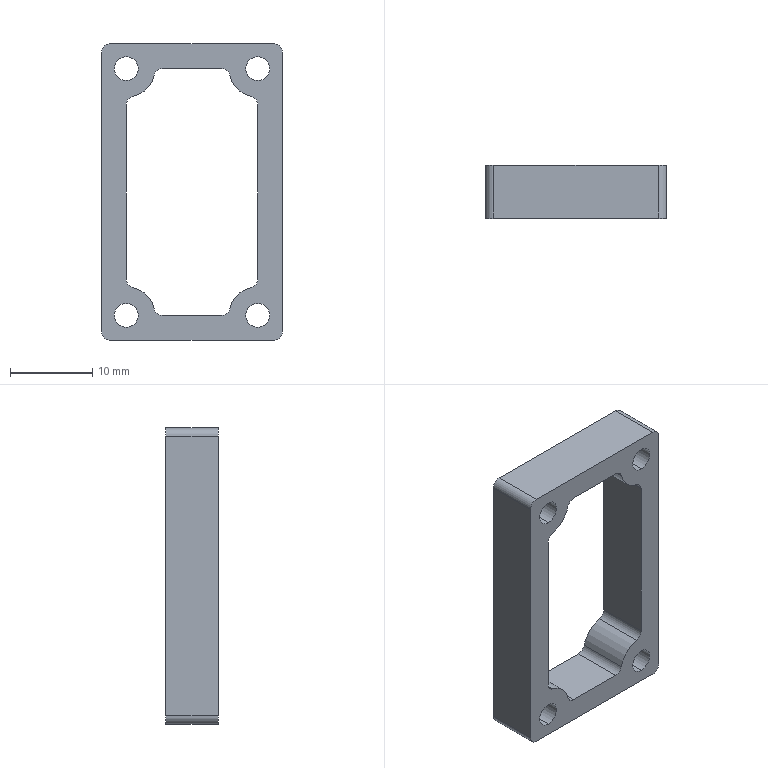Part | SolidWorks | features Fillet 2, Extrusion 1 | 1 solid | 34 faces | box 22 x 6.4 x 36 mm | volume 2076 mm3 | cylinder 24 | plane 10 | commonest cylinder face diameters 2 x12 2.9 x8 7 x4
STEP:
#1=CARTESIAN_POINT('',(8.,6.4,13.55));
#2=VERTEX_POINT('',#1);
#3=CARTESIAN_POINT('',(8.,6.4,16.45));
#4=VERTEX_POINT('',#3);
#5=CARTESIAN_POINT('',(8.,6.4,15.));
#6=DIRECTION('',(0.,1.,0.));
#7=DIRECTION('',(0.,0.,1.));
#8=AXIS2_PLACEMENT_3D('',#5,#6,#7);
#9=CIRCLE('',#8,1.45);
#10=EDGE_CURVE('',#2,#4,#9,.T.);
#11=ORIENTED_EDGE('',*,*,#10,.T.);
#12=CARTESIAN_POINT('',(8.,0.,16.45));
#13=VERTEX_POINT('',#12);
#14=CARTESIAN_POINT('',(8.,6.4,16.45));
#15=DIRECTION('',(0.,-1.,0.));
#16=VECTOR('',#15,1000.);
#17=LINE('',#14,#16);
#18=EDGE_CURVE('',#4,#13,#17,.T.);
#19=ORIENTED_EDGE('',*,*,#18,.T.);
#20=CARTESIAN_POINT('',(8.,0.,13.55));
#21=VERTEX_POINT('',#20);
#22=CARTESIAN_POINT('',(8.,0.,15.));
#23=DIRECTION('',(0.,1.,0.));
#24=DIRECTION('',(0.,0.,1.));
#25=AXIS2_PLACEMENT_3D('',#22,#23,#24);
#26=CIRCLE('',#25,1.45);
#27=EDGE_CURVE('',#21,#13,#26,.T.);
#28=ORIENTED_EDGE('',*,*,#27,.F.);
#29=CARTESIAN_POINT('',(8.,6.4,13.55));
#30=DIRECTION('',(0.,-1.,0.));
#31=VECTOR('',#30,1000.);
#32=LINE('',#29,#31);
#33=EDGE_CURVE('',#2,#21,#32,.T.);
#34=ORIENTED_EDGE('',*,*,#33,.F.);
#35=EDGE_LOOP('',(#11,#19,#28,#34));
#36=FACE_OUTER_BOUND('',#35,.T.);
#37=CARTESIAN_POINT('',(8.,6.4,15.));
#38=DIRECTION('',(0.,-1.,0.));
#39=DIRECTION('',(0.,0.,-1.));
#40=AXIS2_PLACEMENT_3D('',#37,#38,#39);
#41=CYLINDRICAL_SURFACE('',#40,1.45);
#42=ADVANCED_FACE('',(#36),#41,.F.);
#43=CARTESIAN_POINT('',(-8.,6.4,13.55));
#44=VERTEX_POINT('',#43);
#45=CARTESIAN_POINT('',(-8.,6.4,16.45));
#46=VERTEX_POINT('',#45);
#47=CARTESIAN_POINT('',(-8.,6.4,15.));
#48=DIRECTION('',(0.,1.,0.));
#49=DIRECTION('',(0.,0.,1.));
#50=AXIS2_PLACEMENT_3D('',#47,#48,#49);
#51=CIRCLE('',#50,1.45);
#52=EDGE_CURVE('',#44,#46,#51,.T.);
#53=ORIENTED_EDGE('',*,*,#52,.T.);
#54=CARTESIAN_POINT('',(-8.,0.,16.45));
#55=VERTEX_POINT('',#54);
#56=CARTESIAN_POINT('',(-8.,6.4,16.45));
#57=DIRECTION('',(0.,-1.,0.));
#58=VECTOR('',#57,1000.);
#59=LINE('',#56,#58);
#60=EDGE_CURVE('',#46,#55,#59,.T.);
#61=ORIENTED_EDGE('',*,*,#60,.T.);
#62=CARTESIAN_POINT('',(-8.,0.,13.55));
#63=VERTEX_POINT('',#62);
#64=CARTESIAN_POINT('',(-8.,0.,15.));
#65=DIRECTION('',(0.,1.,0.));
#66=DIRECTION('',(0.,0.,1.));
#67=AXIS2_PLACEMENT_3D('',#64,#65,#66);
#68=CIRCLE('',#67,1.45);
#69=EDGE_CURVE('',#63,#55,#68,.T.);
#70=ORIENTED_EDGE('',*,*,#69,.F.);
#71=CARTESIAN_POINT('',(-8.,6.4,13.55));
#72=DIRECTION('',(0.,-1.,0.));
#73=VECTOR('',#72,1000.);
#74=LINE('',#71,#73);
#75=EDGE_CURVE('',#44,#63,#74,.T.);
#76=ORIENTED_EDGE('',*,*,#75,.F.);
#77=EDGE_LOOP('',(#53,#61,#70,#76));
#78=FACE_OUTER_BOUND('',#77,.T.);
#79=CARTESIAN_POINT('',(-8.,6.4,15.));
#80=DIRECTION('',(0.,-1.,0.));
#81=DIRECTION('',(0.,0.,-1.));
#82=AXIS2_PLACEMENT_3D('',#79,#80,#81);
#83=CYLINDRICAL_SURFACE('',#82,1.45);
#84=ADVANCED_FACE('',(#78),#83,.F.);
#85=CARTESIAN_POINT('',(8.,6.4,-16.45));
#86=VERTEX_POINT('',#85);
#87=CARTESIAN_POINT('',(8.,6.4,-13.55));
#88=VERTEX_POINT('',#87);
#89=CARTESIAN_POINT('',(8.,6.4,-15.));
#90=DIRECTION('',(0.,1.,0.));
#91=DIRECTION('',(0.,0.,1.));
#92=AXIS2_PLACEMENT_3D('',#89,#90,#91);
#93=CIRCLE('',#92,1.45);
#94=EDGE_CURVE('',#86,#88,#93,.T.);
#95=ORIENTED_EDGE('',*,*,#94,.T.);
#96=CARTESIAN_POINT('',(8.,0.,-13.55));
#97=VERTEX_POINT('',#96);
#98=CARTESIAN_POINT('',(8.,6.4,-13.55));
#99=DIRECTION('',(0.,-1.,0.));
#100=VECTOR('',#99,1000.);
#101=LINE('',#98,#100);
#102=EDGE_CURVE('',#88,#97,#101,.T.);
#103=ORIENTED_EDGE('',*,*,#102,.T.);
#104=CARTESIAN_POINT('',(8.,0.,-16.45));
#105=VERTEX_POINT('',#104);
#106=CARTESIAN_POINT('',(8.,0.,-15.));
#107=DIRECTION('',(0.,1.,0.));
#108=DIRECTION('',(0.,0.,1.));
#109=AXIS2_PLACEMENT_3D('',#106,#107,#108);
#110=CIRCLE('',#109,1.45);
#111=EDGE_CURVE('',#105,#97,#110,.T.);
#112=ORIENTED_EDGE('',*,*,#111,.F.);
#113=CARTESIAN_POINT('',(8.,6.4,-16.45));
#114=DIRECTION('',(0.,-1.,0.));
#115=VECTOR('',#114,1000.);
#116=LINE('',#113,#115);
#117=EDGE_CURVE('',#86,#105,#116,.T.);
#118=ORIENTED_EDGE('',*,*,#117,.F.);
#119=EDGE_LOOP('',(#95,#103,#112,#118));
#120=FACE_OUTER_BOUND('',#119,.T.);
#121=CARTESIAN_POINT('',(8.,6.4,-15.));
#122=DIRECTION('',(0.,-1.,0.));
#123=DIRECTION('',(0.,0.,-1.));
#124=AXIS2_PLACEMENT_3D('',#121,#122,#123);
#125=CYLINDRICAL_SURFACE('',#124,1.45);
#126=ADVANCED_FACE('',(#120),#125,.F.);
#127=CARTESIAN_POINT('',(-8.,6.4,-16.45));
#128=VERTEX_POINT('',#127);
#129=CARTESIAN_POINT('',(-8.,6.4,-13.55));
#130=VERTEX_POINT('',#129);
#131=CARTESIAN_POINT('',(-8.,6.4,-15.));
#132=DIRECTION('',(0.,1.,0.));
#133=DIRECTION('',(0.,0.,1.));
#134=AXIS2_PLACEMENT_3D('',#131,#132,#133);
#135=CIRCLE('',#134,1.45);
#136=EDGE_CURVE('',#128,#130,#135,.T.);
#137=ORIENTED_EDGE('',*,*,#136,.T.);
#138=CARTESIAN_POINT('',(-8.,0.,-13.55));
#139=VERTEX_POINT('',#138);
#140=CARTESIAN_POINT('',(-8.,6.4,-13.55));
#141=DIRECTION('',(0.,-1.,0.));
#142=VECTOR('',#141,1000.);
#143=LINE('',#140,#142);
#144=EDGE_CURVE('',#130,#139,#143,.T.);
#145=ORIENTED_EDGE('',*,*,#144,.T.);
#146=CARTESIAN_POINT('',(-8.,0.,-16.45));
#147=VERTEX_POINT('',#146);
#148=CARTESIAN_POINT('',(-8.,0.,-15.));
#149=DIRECTION('',(0.,1.,0.));
#150=DIRECTION('',(0.,0.,1.));
#151=AXIS2_PLACEMENT_3D('',#148,#149,#150);
#152=CIRCLE('',#151,1.45);
#153=EDGE_CURVE('',#147,#139,#152,.T.);
#154=ORIENTED_EDGE('',*,*,#153,.F.);
#155=CARTESIAN_POINT('',(-8.,6.4,-16.45));
#156=DIRECTION('',(0.,-1.,0.));
#157=VECTOR('',#156,1000.);
#158=LINE('',#155,#157);
#159=EDGE_CURVE('',#128,#147,#158,.T.);
#160=ORIENTED_EDGE('',*,*,#159,.F.);
#161=EDGE_LOOP('',(#137,#145,#154,#160));
#162=FACE_OUTER_BOUND('',#161,.T.);
#163=CARTESIAN_POINT('',(-8.,6.4,-15.));
#164=DIRECTION('',(0.,-1.,0.));
#165=DIRECTION('',(0.,0.,-1.));
#166=AXIS2_PLACEMENT_3D('',#163,#164,#165);
#167=CYLINDRICAL_SURFACE('',#166,1.45);
#168=ADVANCED_FACE('',(#162),#167,.F.);
#169=CARTESIAN_POINT('',(8.,0.,-10.613));
#170=VERTEX_POINT('',#169);
#171=CARTESIAN_POINT('',(8.,0.,10.613));
#172=VERTEX_POINT('',#171);
#173=CARTESIAN_POINT('',(8.,0.,0.));
#174=DIRECTION('',(0.,0.,1.));
#175=VECTOR('',#174,1000.);
#176=LINE('',#173,#175);
#177=EDGE_CURVE('',#170,#172,#176,.T.);
#178=ORIENTED_EDGE('',*,*,#177,.T.);
#179=CARTESIAN_POINT('',(8.,6.4,10.613));
#180=VERTEX_POINT('',#179);
#181=CARTESIAN_POINT('',(8.,6.4,10.613));
#182=DIRECTION('',(0.,1.,0.));
#183=VECTOR('',#182,1000.);
#184=LINE('',#181,#183);
#185=EDGE_CURVE('',#172,#180,#184,.T.);
#186=ORIENTED_EDGE('',*,*,#185,.T.);
#187=CARTESIAN_POINT('',(8.,6.4,-10.613));
#188=VERTEX_POINT('',#187);
#189=CARTESIAN_POINT('',(8.,6.4,0.));
#190=DIRECTION('',(0.,0.,1.));
#191=VECTOR('',#190,1000.);
#192=LINE('',#189,#191);
#193=EDGE_CURVE('',#188,#180,#192,.T.);
#194=ORIENTED_EDGE('',*,*,#193,.F.);
#195=CARTESIAN_POINT('',(8.,0.,-10.613));
#196=DIRECTION('',(0.,-1.,0.));
#197=VECTOR('',#196,1000.);
#198=LINE('',#195,#197);
#199=EDGE_CURVE('',#188,#170,#198,.T.);
#200=ORIENTED_EDGE('',*,*,#199,.T.);
#201=EDGE_LOOP('',(#178,#186,#194,#200));
#202=FACE_OUTER_BOUND('',#201,.T.);
#203=CARTESIAN_POINT('',(8.,6.4,0.));
#204=DIRECTION('',(1.,0.,0.));
#205=DIRECTION('',(0.,0.,-1.));
#206=AXIS2_PLACEMENT_3D('',#203,#204,#205);
#207=PLANE('',#206);
#208=ADVANCED_FACE('',(#202),#207,.F.);
#209=CARTESIAN_POINT('',(7.222,0.,11.588));
#210=VERTEX_POINT('',#209);
#211=CARTESIAN_POINT('',(4.588,0.,14.222));
#212=VERTEX_POINT('',#211);
#213=CARTESIAN_POINT('',(8.,0.,15.));
#214=DIRECTION('',(0.,1.,0.));
#215=DIRECTION('',(0.,0.,1.));
#216=AXIS2_PLACEMENT_3D('',#213,#214,#215);
#217=CIRCLE('',#216,3.5);
#218=EDGE_CURVE('',#210,#212,#217,.T.);
#219=ORIENTED_EDGE('',*,*,#218,.T.);
#220=CARTESIAN_POINT('',(4.588,6.4,14.222));
#221=VERTEX_POINT('',#220);
#222=CARTESIAN_POINT('',(4.588,6.4,14.222));
#223=DIRECTION('',(0.,1.,0.));
#224=VECTOR('',#223,1000.);
#225=LINE('',#222,#224);
#226=EDGE_CURVE('',#212,#221,#225,.T.);
#227=ORIENTED_EDGE('',*,*,#226,.T.);
#228=CARTESIAN_POINT('',(7.222,6.4,11.588));
#229=VERTEX_POINT('',#228);
#230=CARTESIAN_POINT('',(8.,6.4,15.));
#231=DIRECTION('',(0.,1.,0.));
#232=DIRECTION('',(0.,0.,1.));
#233=AXIS2_PLACEMENT_3D('',#230,#231,#232);
#234=CIRCLE('',#233,3.5);
#235=EDGE_CURVE('',#229,#221,#234,.T.);
#236=ORIENTED_EDGE('',*,*,#235,.F.);
#237=CARTESIAN_POINT('',(7.222,6.4,11.588));
#238=DIRECTION('',(0.,-1.,0.));
#239=VECTOR('',#238,1000.);
#240=LINE('',#237,#239);
#241=EDGE_CURVE('',#229,#210,#240,.T.);
#242=ORIENTED_EDGE('',*,*,#241,.T.);
#243=EDGE_LOOP('',(#219,#227,#236,#242));
#244=FACE_OUTER_BOUND('',#243,.T.);
#245=CARTESIAN_POINT('',(8.,6.4,15.));
#246=DIRECTION('',(0.,-1.,0.));
#247=DIRECTION('',(0.,0.,-1.));
#248=AXIS2_PLACEMENT_3D('',#245,#246,#247);
#249=CYLINDRICAL_SURFACE('',#248,3.5);
#250=ADVANCED_FACE('',(#244),#249,.T.);
#251=CARTESIAN_POINT('',(-3.613,0.,15.));
#252=VERTEX_POINT('',#251);
#253=CARTESIAN_POINT('',(3.613,0.,15.));
#254=VERTEX_POINT('',#253);
#255=CARTESIAN_POINT('',(0.,0.,15.));
#256=DIRECTION('',(1.,0.,0.));
#257=VECTOR('',#256,1000.);
#258=LINE('',#255,#257);
#259=EDGE_CURVE('',#252,#254,#258,.T.);
#260=ORIENTED_EDGE('',*,*,#259,.F.);
#261=CARTESIAN_POINT('',(-3.613,6.4,15.));
#262=VERTEX_POINT('',#261);
#263=CARTESIAN_POINT('',(-3.613,6.4,15.));
#264=DIRECTION('',(0.,1.,0.));
#265=VECTOR('',#264,1000.);
#266=LINE('',#263,#265);
#267=EDGE_CURVE('',#252,#262,#266,.T.);
#268=ORIENTED_EDGE('',*,*,#267,.T.);
#269=CARTESIAN_POINT('',(3.613,6.4,15.));
#270=VERTEX_POINT('',#269);
#271=CARTESIAN_POINT('',(0.,6.4,15.));
#272=DIRECTION('',(1.,0.,0.));
#273=VECTOR('',#272,1000.);
#274=LINE('',#271,#273);
#275=EDGE_CURVE('',#262,#270,#274,.T.);
#276=ORIENTED_EDGE('',*,*,#275,.T.);
#277=CARTESIAN_POINT('',(3.613,6.4,15.));
#278=DIRECTION('',(0.,-1.,0.));
#279=VECTOR('',#278,1000.);
#280=LINE('',#277,#279);
#281=EDGE_CURVE('',#270,#254,#280,.T.);
#282=ORIENTED_EDGE('',*,*,#281,.T.);
#283=EDGE_LOOP('',(#260,#268,#276,#282));
#284=FACE_OUTER_BOUND('',#283,.T.);
#285=CARTESIAN_POINT('',(0.,6.4,15.));
#286=DIRECTION('',(0.,0.,-1.));
#287=DIRECTION('',(-1.,0.,0.));
#288=AXIS2_PLACEMENT_3D('',#285,#286,#287);
#289=PLANE('',#288);
#290=ADVANCED_FACE('',(#284),#289,.T.);
#291=CARTESIAN_POINT('',(-7.222,6.4,11.588));
#292=VERTEX_POINT('',#291);
#293=CARTESIAN_POINT('',(-4.588,6.4,14.222));
#294=VERTEX_POINT('',#293);
#295=CARTESIAN_POINT('',(-8.,6.4,15.));
#296=DIRECTION('',(0.,-1.,0.));
#297=DIRECTION('',(0.,0.,1.));
#298=AXIS2_PLACEMENT_3D('',#295,#296,#297);
#299=CIRCLE('',#298,3.5);
#300=EDGE_CURVE('',#292,#294,#299,.T.);
#301=ORIENTED_EDGE('',*,*,#300,.T.);
#302=CARTESIAN_POINT('',(-4.588,0.,14.222));
#303=VERTEX_POINT('',#302);
#304=CARTESIAN_POINT('',(-4.588,6.4,14.222));
#305=DIRECTION('',(0.,-1.,0.));
#306=VECTOR('',#305,1000.);
#307=LINE('',#304,#306);
#308=EDGE_CURVE('',#294,#303,#307,.T.);
#309=ORIENTED_EDGE('',*,*,#308,.T.);
#310=CARTESIAN_POINT('',(-7.222,0.,11.588));
#311=VERTEX_POINT('',#310);
#312=CARTESIAN_POINT('',(-8.,0.,15.));
#313=DIRECTION('',(0.,-1.,0.));
#314=DIRECTION('',(0.,0.,1.));
#315=AXIS2_PLACEMENT_3D('',#312,#313,#314);
#316=CIRCLE('',#315,3.5);
#317=EDGE_CURVE('',#311,#303,#316,.T.);
#318=ORIENTED_EDGE('',*,*,#317,.F.);
#319=CARTESIAN_POINT('',(-7.222,6.4,11.588));
#320=DIRECTION('',(0.,1.,0.));
#321=VECTOR('',#320,1000.);
#322=LINE('',#319,#321);
#323=EDGE_CURVE('',#311,#292,#322,.T.);
#324=ORIENTED_EDGE('',*,*,#323,.T.);
#325=EDGE_LOOP('',(#301,#309,#318,#324));
#326=FACE_OUTER_BOUND('',#325,.T.);
#327=CARTESIAN_POINT('',(-8.,6.4,15.));
#328=DIRECTION('',(0.,-1.,0.));
#329=DIRECTION('',(0.,0.,-1.));
#330=AXIS2_PLACEMENT_3D('',#327,#328,#329);
#331=CYLINDRICAL_SURFACE('',#330,3.5);
#332=ADVANCED_FACE('',(#326),#331,.T.);
#333=CARTESIAN_POINT('',(-8.,6.4,-10.613));
#334=VERTEX_POINT('',#333);
#335=CARTESIAN_POINT('',(-8.,6.4,10.613));
#336=VERTEX_POINT('',#335);
#337=CARTESIAN_POINT('',(-8.,6.4,0.));
#338=DIRECTION('',(0.,0.,1.));
#339=VECTOR('',#338,1000.);
#340=LINE('',#337,#339);
#341=EDGE_CURVE('',#334,#336,#340,.T.);
#342=ORIENTED_EDGE('',*,*,#341,.T.);
#343=CARTESIAN_POINT('',(-8.,0.,10.613));
#344=VERTEX_POINT('',#343);
#345=CARTESIAN_POINT('',(-8.,0.,10.613));
#346=DIRECTION('',(0.,-1.,0.));
#347=VECTOR('',#346,1000.);
#348=LINE('',#345,#347);
#349=EDGE_CURVE('',#336,#344,#348,.T.);
#350=ORIENTED_EDGE('',*,*,#349,.T.);
#351=CARTESIAN_POINT('',(-8.,0.,-10.613));
#352=VERTEX_POINT('',#351);
#353=CARTESIAN_POINT('',(-8.,0.,0.));
#354=DIRECTION('',(0.,0.,1.));
#355=VECTOR('',#354,1000.);
#356=LINE('',#353,#355);
#357=EDGE_CURVE('',#352,#344,#356,.T.);
#358=ORIENTED_EDGE('',*,*,#357,.F.);
#359=CARTESIAN_POINT('',(-8.,6.4,-10.613));
#360=DIRECTION('',(0.,1.,0.));
#361=VECTOR('',#360,1000.);
#362=LINE('',#359,#361);
#363=EDGE_CURVE('',#352,#334,#362,.T.);
#364=ORIENTED_EDGE('',*,*,#363,.T.);
#365=EDGE_LOOP('',(#342,#350,#358,#364));
#366=FACE_OUTER_BOUND('',#365,.T.);
#367=CARTESIAN_POINT('',(-8.,6.4,0.));
#368=DIRECTION('',(1.,0.,0.));
#369=DIRECTION('',(0.,0.,-1.));
#370=AXIS2_PLACEMENT_3D('',#367,#368,#369);
#371=PLANE('',#370);
#372=ADVANCED_FACE('',(#366),#371,.T.);
#373=CARTESIAN_POINT('',(-4.588,6.4,-14.222));
#374=VERTEX_POINT('',#373);
#375=CARTESIAN_POINT('',(-7.222,6.4,-11.588));
#376=VERTEX_POINT('',#375);
#377=CARTESIAN_POINT('',(-8.,6.4,-15.));
#378=DIRECTION('',(0.,-1.,0.));
#379=DIRECTION('',(0.,0.,1.));
#380=AXIS2_PLACEMENT_3D('',#377,#378,#379);
#381=CIRCLE('',#380,3.5);
#382=EDGE_CURVE('',#374,#376,#381,.T.);
#383=ORIENTED_EDGE('',*,*,#382,.T.);
#384=CARTESIAN_POINT('',(-7.222,0.,-11.588));
#385=VERTEX_POINT('',#384);
#386=CARTESIAN_POINT('',(-7.222,6.4,-11.588));
#387=DIRECTION('',(0.,-1.,0.));
#388=VECTOR('',#387,1000.);
#389=LINE('',#386,#388);
#390=EDGE_CURVE('',#376,#385,#389,.T.);
#391=ORIENTED_EDGE('',*,*,#390,.T.);
#392=CARTESIAN_POINT('',(-4.588,0.,-14.222));
#393=VERTEX_POINT('',#392);
#394=CARTESIAN_POINT('',(-8.,0.,-15.));
#395=DIRECTION('',(0.,-1.,0.));
#396=DIRECTION('',(0.,0.,1.));
#397=AXIS2_PLACEMENT_3D('',#394,#395,#396);
#398=CIRCLE('',#397,3.5);
#399=EDGE_CURVE('',#393,#385,#398,.T.);
#400=ORIENTED_EDGE('',*,*,#399,.F.);
#401=CARTESIAN_POINT('',(-4.588,6.4,-14.222));
#402=DIRECTION('',(0.,1.,0.));
#403=VECTOR('',#402,1000.);
#404=LINE('',#401,#403);
#405=EDGE_CURVE('',#393,#374,#404,.T.);
#406=ORIENTED_EDGE('',*,*,#405,.T.);
#407=EDGE_LOOP('',(#383,#391,#400,#406));
#408=FACE_OUTER_BOUND('',#407,.T.);
#409=CARTESIAN_POINT('',(-8.,6.4,-15.));
#410=DIRECTION('',(0.,-1.,0.));
#411=DIRECTION('',(0.,0.,-1.));
#412=AXIS2_PLACEMENT_3D('',#409,#410,#411);
#413=CYLINDRICAL_SURFACE('',#412,3.5);
#414=ADVANCED_FACE('',(#408),#413,.T.);
#415=CARTESIAN_POINT('',(-3.613,0.,-15.));
#416=VERTEX_POINT('',#415);
#417=CARTESIAN_POINT('',(3.613,0.,-15.));
#418=VERTEX_POINT('',#417);
#419=CARTESIAN_POINT('',(0.,0.,-15.));
#420=DIRECTION('',(1.,0.,0.));
#421=VECTOR('',#420,1000.);
#422=LINE('',#419,#421);
#423=EDGE_CURVE('',#416,#418,#422,.T.);
#424=ORIENTED_EDGE('',*,*,#423,.T.);
#425=CARTESIAN_POINT('',(3.613,6.4,-15.));
#426=VERTEX_POINT('',#425);
#427=CARTESIAN_POINT('',(3.613,6.4,-15.));
#428=DIRECTION('',(0.,1.,0.));
#429=VECTOR('',#428,1000.);
#430=LINE('',#427,#429);
#431=EDGE_CURVE('',#418,#426,#430,.T.);
#432=ORIENTED_EDGE('',*,*,#431,.T.);
#433=CARTESIAN_POINT('',(-3.613,6.4,-15.));
#434=VERTEX_POINT('',#433);
#435=CARTESIAN_POINT('',(0.,6.4,-15.));
#436=DIRECTION('',(1.,0.,0.));
#437=VECTOR('',#436,1000.);
#438=LINE('',#435,#437);
#439=EDGE_CURVE('',#434,#426,#438,.T.);
#440=ORIENTED_EDGE('',*,*,#439,.F.);
#441=CARTESIAN_POINT('',(-3.613,6.4,-15.));
#442=DIRECTION('',(0.,-1.,0.));
#443=VECTOR('',#442,1000.);
#444=LINE('',#441,#443);
#445=EDGE_CURVE('',#434,#416,#444,.T.);
#446=ORIENTED_EDGE('',*,*,#445,.T.);
#447=EDGE_LOOP('',(#424,#432,#440,#446));
#448=FACE_OUTER_BOUND('',#447,.T.);
#449=CARTESIAN_POINT('',(0.,6.4,-15.));
#450=DIRECTION('',(0.,0.,-1.));
#451=DIRECTION('',(-1.,0.,0.));
#452=AXIS2_PLACEMENT_3D('',#449,#450,#451);
#453=PLANE('',#452);
#454=ADVANCED_FACE('',(#448),#453,.F.);
#455=CARTESIAN_POINT('',(-11.,0.,17.));
#456=VERTEX_POINT('',#455);
#457=CARTESIAN_POINT('',(-11.,0.,-17.));
#458=VERTEX_POINT('',#457);
#459=CARTESIAN_POINT('',(-11.,0.,0.));
#460=DIRECTION('',(0.,0.,-1.));
#461=VECTOR('',#460,1000.);
#462=LINE('',#459,#461);
#463=EDGE_CURVE('',#456,#458,#462,.T.);
#464=ORIENTED_EDGE('',*,*,#463,.F.);
#465=CARTESIAN_POINT('',(-11.,6.4,17.));
#466=VERTEX_POINT('',#465);
#467=CARTESIAN_POINT('',(-11.,6.4,17.));
#468=DIRECTION('',(0.,1.,0.));
#469=VECTOR('',#468,1000.);
#470=LINE('',#467,#469);
#471=EDGE_CURVE('',#456,#466,#470,.T.);
#472=ORIENTED_EDGE('',*,*,#471,.T.);
#473=CARTESIAN_POINT('',(-11.,6.4,-17.));
#474=VERTEX_POINT('',#473);
#475=CARTESIAN_POINT('',(-11.,6.4,0.));
#476=DIRECTION('',(0.,0.,-1.));
#477=VECTOR('',#476,1000.);
#478=LINE('',#475,#477);
#479=EDGE_CURVE('',#466,#474,#478,.T.);
#480=ORIENTED_EDGE('',*,*,#479,.T.);
#481=CARTESIAN_POINT('',(-11.,0.,-17.));
#482=DIRECTION('',(0.,-1.,0.));
#483=VECTOR('',#482,1000.);
#484=LINE('',#481,#483);
#485=EDGE_CURVE('',#474,#458,#484,.T.);
#486=ORIENTED_EDGE('',*,*,#485,.T.);
#487=EDGE_LOOP('',(#464,#472,#480,#486));
#488=FACE_OUTER_BOUND('',#487,.T.);
#489=CARTESIAN_POINT('',(-11.,6.4,0.));
#490=DIRECTION('',(-1.,0.,0.));
#491=DIRECTION('',(0.,0.,1.));
#492=AXIS2_PLACEMENT_3D('',#489,#490,#491);
#493=PLANE('',#492);
#494=ADVANCED_FACE('',(#488),#493,.T.);
#495=CARTESIAN_POINT('',(10.,6.4,18.));
#496=VERTEX_POINT('',#495);
#497=CARTESIAN_POINT('',(-10.,6.4,18.));
#498=VERTEX_POINT('',#497);
#499=CARTESIAN_POINT('',(0.,6.4,18.));
#500=DIRECTION('',(-1.,0.,0.));
#501=VECTOR('',#500,1000.);
#502=LINE('',#499,#501);
#503=EDGE_CURVE('',#496,#498,#502,.T.);
#504=ORIENTED_EDGE('',*,*,#503,.T.);
#505=CARTESIAN_POINT('',(-10.,0.,18.));
#506=VERTEX_POINT('',#505);
#507=CARTESIAN_POINT('',(-10.,6.4,18.));
#508=DIRECTION('',(0.,-1.,0.));
#509=VECTOR('',#508,1000.);
#510=LINE('',#507,#509);
#511=EDGE_CURVE('',#498,#506,#510,.T.);
#512=ORIENTED_EDGE('',*,*,#511,.T.);
#513=CARTESIAN_POINT('',(10.,0.,18.));
#514=VERTEX_POINT('',#513);
#515=CARTESIAN_POINT('',(0.,0.,18.));
#516=DIRECTION('',(-1.,0.,0.));
#517=VECTOR('',#516,1000.);
#518=LINE('',#515,#517);
#519=EDGE_CURVE('',#514,#506,#518,.T.);
#520=ORIENTED_EDGE('',*,*,#519,.F.);
#521=CARTESIAN_POINT('',(10.,6.4,18.));
#522=DIRECTION('',(0.,1.,0.));
#523=VECTOR('',#522,1000.);
#524=LINE('',#521,#523);
#525=EDGE_CURVE('',#514,#496,#524,.T.);
#526=ORIENTED_EDGE('',*,*,#525,.T.);
#527=EDGE_LOOP('',(#504,#512,#520,#526));
#528=FACE_OUTER_BOUND('',#527,.T.);
#529=CARTESIAN_POINT('',(0.,6.4,18.));
#530=DIRECTION('',(0.,0.,1.));
#531=DIRECTION('',(1.,0.,0.));
#532=AXIS2_PLACEMENT_3D('',#529,#530,#531);
#533=PLANE('',#532);
#534=ADVANCED_FACE('',(#528),#533,.T.);
#535=CARTESIAN_POINT('',(11.,6.4,17.));
#536=VERTEX_POINT('',#535);
#537=CARTESIAN_POINT('',(11.,6.4,-17.));
#538=VERTEX_POINT('',#537);
#539=CARTESIAN_POINT('',(11.,6.4,0.));
#540=DIRECTION('',(0.,0.,-1.));
#541=VECTOR('',#540,1000.);
#542=LINE('',#539,#541);
#543=EDGE_CURVE('',#536,#538,#542,.T.);
#544=ORIENTED_EDGE('',*,*,#543,.F.);
#545=CARTESIAN_POINT('',(11.,0.,17.));
#546=VERTEX_POINT('',#545);
#547=CARTESIAN_POINT('',(11.,0.,17.));
#548=DIRECTION('',(0.,-1.,0.));
#549=VECTOR('',#548,1000.);
#550=LINE('',#547,#549);
#551=EDGE_CURVE('',#536,#546,#550,.T.);
#552=ORIENTED_EDGE('',*,*,#551,.T.);
#553=CARTESIAN_POINT('',(11.,0.,-17.));
#554=VERTEX_POINT('',#553);
#555=CARTESIAN_POINT('',(11.,0.,0.));
#556=DIRECTION('',(0.,0.,-1.));
#557=VECTOR('',#556,1000.);
#558=LINE('',#555,#557);
#559=EDGE_CURVE('',#546,#554,#558,.T.);
#560=ORIENTED_EDGE('',*,*,#559,.T.);
#561=CARTESIAN_POINT('',(11.,6.4,-17.));
#562=DIRECTION('',(0.,1.,0.));
#563=VECTOR('',#562,1000.);
#564=LINE('',#561,#563);
#565=EDGE_CURVE('',#554,#538,#564,.T.);
#566=ORIENTED_EDGE('',*,*,#565,.T.);
#567=EDGE_LOOP('',(#544,#552,#560,#566));
#568=FACE_OUTER_BOUND('',#567,.T.);
#569=CARTESIAN_POINT('',(11.,6.4,0.));
#570=DIRECTION('',(-1.,0.,0.));
#571=DIRECTION('',(0.,0.,1.));
#572=AXIS2_PLACEMENT_3D('',#569,#570,#571);
#573=PLANE('',#572);
#574=ADVANCED_FACE('',(#568),#573,.F.);
#575=CARTESIAN_POINT('',(10.,6.4,-18.));
#576=VERTEX_POINT('',#575);
#577=CARTESIAN_POINT('',(-10.,6.4,-18.));
#578=VERTEX_POINT('',#577);
#579=CARTESIAN_POINT('',(0.,6.4,-18.));
#580=DIRECTION('',(-1.,0.,0.));
#581=VECTOR('',#580,1000.);
#582=LINE('',#579,#581);
#583=EDGE_CURVE('',#576,#578,#582,.T.);
#584=ORIENTED_EDGE('',*,*,#583,.F.);
#585=CARTESIAN_POINT('',(10.,0.,-18.));
#586=VERTEX_POINT('',#585);
#587=CARTESIAN_POINT('',(10.,6.4,-18.));
#588=DIRECTION('',(0.,-1.,0.));
#589=VECTOR('',#588,1000.);
#590=LINE('',#587,#589);
#591=EDGE_CURVE('',#576,#586,#590,.T.);
#592=ORIENTED_EDGE('',*,*,#591,.T.);
#593=CARTESIAN_POINT('',(-10.,0.,-18.));
#594=VERTEX_POINT('',#593);
#595=CARTESIAN_POINT('',(0.,0.,-18.));
#596=DIRECTION('',(-1.,0.,0.));
#597=VECTOR('',#596,1000.);
#598=LINE('',#595,#597);
#599=EDGE_CURVE('',#586,#594,#598,.T.);
#600=ORIENTED_EDGE('',*,*,#599,.T.);
#601=CARTESIAN_POINT('',(-10.,6.4,-18.));
#602=DIRECTION('',(0.,1.,0.));
#603=VECTOR('',#602,1000.);
#604=LINE('',#601,#603);
#605=EDGE_CURVE('',#594,#578,#604,.T.);
#606=ORIENTED_EDGE('',*,*,#605,.T.);
#607=EDGE_LOOP('',(#584,#592,#600,#606));
#608=FACE_OUTER_BOUND('',#607,.T.);
#609=CARTESIAN_POINT('',(0.,6.4,-18.));
#610=DIRECTION('',(0.,0.,1.));
#611=DIRECTION('',(1.,0.,0.));
#612=AXIS2_PLACEMENT_3D('',#609,#610,#611);
#613=PLANE('',#612);
#614=ADVANCED_FACE('',(#608),#613,.F.);
#615=ORIENTED_EDGE('',*,*,#144,.F.);
#616=CARTESIAN_POINT('',(-8.,6.4,-15.));
#617=DIRECTION('',(0.,1.,0.));
#618=DIRECTION('',(0.,0.,1.));
#619=AXIS2_PLACEMENT_3D('',#616,#617,#618);
#620=CIRCLE('',#619,1.45);
#621=EDGE_CURVE('',#130,#128,#620,.T.);
#622=ORIENTED_EDGE('',*,*,#621,.T.);
#623=ORIENTED_EDGE('',*,*,#159,.T.);
#624=CARTESIAN_POINT('',(-8.,0.,-15.));
#625=DIRECTION('',(0.,1.,0.));
#626=DIRECTION('',(0.,0.,1.));
#627=AXIS2_PLACEMENT_3D('',#624,#625,#626);
#628=CIRCLE('',#627,1.45);
#629=EDGE_CURVE('',#139,#147,#628,.T.);
#630=ORIENTED_EDGE('',*,*,#629,.F.);
#631=EDGE_LOOP('',(#615,#622,#623,#630));
#632=FACE_OUTER_BOUND('',#631,.T.);
#633=CARTESIAN_POINT('',(-8.,6.4,-15.));
#634=DIRECTION('',(0.,-1.,0.));
#635=DIRECTION('',(0.,0.,-1.));
#636=AXIS2_PLACEMENT_3D('',#633,#634,#635);
#637=CYLINDRICAL_SURFACE('',#636,1.45);
#638=ADVANCED_FACE('',(#632),#637,.F.);
#639=ORIENTED_EDGE('',*,*,#102,.F.);
#640=CARTESIAN_POINT('',(8.,6.4,-15.));
#641=DIRECTION('',(0.,1.,0.));
#642=DIRECTION('',(0.,0.,1.));
#643=AXIS2_PLACEMENT_3D('',#640,#641,#642);
#644=CIRCLE('',#643,1.45);
#645=EDGE_CURVE('',#88,#86,#644,.T.);
#646=ORIENTED_EDGE('',*,*,#645,.T.);
#647=ORIENTED_EDGE('',*,*,#117,.T.);
#648=CARTESIAN_POINT('',(8.,0.,-15.));
#649=DIRECTION('',(0.,1.,0.));
#650=DIRECTION('',(0.,0.,1.));
#651=AXIS2_PLACEMENT_3D('',#648,#649,#650);
#652=CIRCLE('',#651,1.45);
#653=EDGE_CURVE('',#97,#105,#652,.T.);
#654=ORIENTED_EDGE('',*,*,#653,.F.);
#655=EDGE_LOOP('',(#639,#646,#647,#654));
#656=FACE_OUTER_BOUND('',#655,.T.);
#657=CARTESIAN_POINT('',(8.,6.4,-15.));
#658=DIRECTION('',(0.,-1.,0.));
#659=DIRECTION('',(0.,0.,-1.));
#660=AXIS2_PLACEMENT_3D('',#657,#658,#659);
#661=CYLINDRICAL_SURFACE('',#660,1.45);
#662=ADVANCED_FACE('',(#656),#661,.F.);
#663=ORIENTED_EDGE('',*,*,#60,.F.);
#664=CARTESIAN_POINT('',(-8.,6.4,15.));
#665=DIRECTION('',(0.,1.,0.));
#666=DIRECTION('',(0.,0.,1.));
#667=AXIS2_PLACEMENT_3D('',#664,#665,#666);
#668=CIRCLE('',#667,1.45);
#669=EDGE_CURVE('',#46,#44,#668,.T.);
#670=ORIENTED_EDGE('',*,*,#669,.T.);
#671=ORIENTED_EDGE('',*,*,#75,.T.);
#672=CARTESIAN_POINT('',(-8.,0.,15.));
#673=DIRECTION('',(0.,1.,0.));
#674=DIRECTION('',(0.,0.,1.));
#675=AXIS2_PLACEMENT_3D('',#672,#673,#674);
#676=CIRCLE('',#675,1.45);
#677=EDGE_CURVE('',#55,#63,#676,.T.);
#678=ORIENTED_EDGE('',*,*,#677,.F.);
#679=EDGE_LOOP('',(#663,#670,#671,#678));
#680=FACE_OUTER_BOUND('',#679,.T.);
#681=CARTESIAN_POINT('',(-8.,6.4,15.));
#682=DIRECTION('',(0.,-1.,0.));
#683=DIRECTION('',(0.,0.,-1.));
#684=AXIS2_PLACEMENT_3D('',#681,#682,#683);
#685=CYLINDRICAL_SURFACE('',#684,1.45);
#686=ADVANCED_FACE('',(#680),#685,.F.);
#687=ORIENTED_EDGE('',*,*,#18,.F.);
#688=CARTESIAN_POINT('',(8.,6.4,15.));
#689=DIRECTION('',(0.,1.,0.));
#690=DIRECTION('',(0.,0.,1.));
#691=AXIS2_PLACEMENT_3D('',#688,#689,#690);
#692=CIRCLE('',#691,1.45);
#693=EDGE_CURVE('',#4,#2,#692,.T.);
#694=ORIENTED_EDGE('',*,*,#693,.T.);
#695=ORIENTED_EDGE('',*,*,#33,.T.);
#696=CARTESIAN_POINT('',(8.,0.,15.));
#697=DIRECTION('',(0.,1.,0.));
#698=DIRECTION('',(0.,0.,1.));
#699=AXIS2_PLACEMENT_3D('',#696,#697,#698);
#700=CIRCLE('',#699,1.45);
#701=EDGE_CURVE('',#13,#21,#700,.T.);
#702=ORIENTED_EDGE('',*,*,#701,.F.);
#703=EDGE_LOOP('',(#687,#694,#695,#702));
#704=FACE_OUTER_BOUND('',#703,.T.);
#705=CARTESIAN_POINT('',(8.,6.4,15.));
#706=DIRECTION('',(0.,-1.,0.));
#707=DIRECTION('',(0.,0.,-1.));
#708=AXIS2_PLACEMENT_3D('',#705,#706,#707);
#709=CYLINDRICAL_SURFACE('',#708,1.45);
#710=ADVANCED_FACE('',(#704),#709,.F.);
#711=CARTESIAN_POINT('',(4.588,0.,-14.222));
#712=VERTEX_POINT('',#711);
#713=CARTESIAN_POINT('',(7.222,0.,-11.588));
#714=VERTEX_POINT('',#713);
#715=CARTESIAN_POINT('',(8.,0.,-15.));
#716=DIRECTION('',(0.,1.,0.));
#717=DIRECTION('',(0.,0.,1.));
#718=AXIS2_PLACEMENT_3D('',#715,#716,#717);
#719=CIRCLE('',#718,3.5);
#720=EDGE_CURVE('',#712,#714,#719,.T.);
#721=ORIENTED_EDGE('',*,*,#720,.T.);
#722=CARTESIAN_POINT('',(7.222,6.4,-11.588));
#723=VERTEX_POINT('',#722);
#724=CARTESIAN_POINT('',(7.222,6.4,-11.588));
#725=DIRECTION('',(0.,1.,0.));
#726=VECTOR('',#725,1000.);
#727=LINE('',#724,#726);
#728=EDGE_CURVE('',#714,#723,#727,.T.);
#729=ORIENTED_EDGE('',*,*,#728,.T.);
#730=CARTESIAN_POINT('',(4.588,6.4,-14.222));
#731=VERTEX_POINT('',#730);
#732=CARTESIAN_POINT('',(8.,6.4,-15.));
#733=DIRECTION('',(0.,1.,0.));
#734=DIRECTION('',(0.,0.,1.));
#735=AXIS2_PLACEMENT_3D('',#732,#733,#734);
#736=CIRCLE('',#735,3.5);
#737=EDGE_CURVE('',#731,#723,#736,.T.);
#738=ORIENTED_EDGE('',*,*,#737,.F.);
#739=CARTESIAN_POINT('',(4.588,6.4,-14.222));
#740=DIRECTION('',(0.,-1.,0.));
#741=VECTOR('',#740,1000.);
#742=LINE('',#739,#741);
#743=EDGE_CURVE('',#731,#712,#742,.T.);
#744=ORIENTED_EDGE('',*,*,#743,.T.);
#745=EDGE_LOOP('',(#721,#729,#738,#744));
#746=FACE_OUTER_BOUND('',#745,.T.);
#747=CARTESIAN_POINT('',(8.,6.4,-15.));
#748=DIRECTION('',(0.,-1.,0.));
#749=DIRECTION('',(0.,0.,-1.));
#750=AXIS2_PLACEMENT_3D('',#747,#748,#749);
#751=CYLINDRICAL_SURFACE('',#750,3.5);
#752=ADVANCED_FACE('',(#746),#751,.T.);
#753=ORIENTED_EDGE('',*,*,#10,.F.);
#754=ORIENTED_EDGE('',*,*,#693,.F.);
#755=EDGE_LOOP('',(#753,#754));
#756=FACE_BOUND('',#755,.T.);
#757=ORIENTED_EDGE('',*,*,#52,.F.);
#758=ORIENTED_EDGE('',*,*,#669,.F.);
#759=EDGE_LOOP('',(#757,#758));
#760=FACE_BOUND('',#759,.T.);
#761=ORIENTED_EDGE('',*,*,#94,.F.);
#762=ORIENTED_EDGE('',*,*,#645,.F.);
#763=EDGE_LOOP('',(#761,#762));
#764=FACE_BOUND('',#763,.T.);
#765=ORIENTED_EDGE('',*,*,#136,.F.);
#766=ORIENTED_EDGE('',*,*,#621,.F.);
#767=EDGE_LOOP('',(#765,#766));
#768=FACE_BOUND('',#767,.T.);
#769=ORIENTED_EDGE('',*,*,#479,.F.);
#770=CARTESIAN_POINT('',(-10.,6.4,17.));
#771=DIRECTION('',(0.,1.,0.));
#772=DIRECTION('',(0.,0.,1.));
#773=AXIS2_PLACEMENT_3D('',#770,#771,#772);
#774=CIRCLE('',#773,1.);
#775=EDGE_CURVE('',#466,#498,#774,.T.);
#776=ORIENTED_EDGE('',*,*,#775,.T.);
#777=ORIENTED_EDGE('',*,*,#503,.F.);
#778=CARTESIAN_POINT('',(10.,6.4,17.));
#779=DIRECTION('',(0.,1.,0.));
#780=DIRECTION('',(0.,0.,1.));
#781=AXIS2_PLACEMENT_3D('',#778,#779,#780);
#782=CIRCLE('',#781,1.);
#783=EDGE_CURVE('',#496,#536,#782,.T.);
#784=ORIENTED_EDGE('',*,*,#783,.T.);
#785=ORIENTED_EDGE('',*,*,#543,.T.);
#786=CARTESIAN_POINT('',(10.,6.4,-17.));
#787=DIRECTION('',(0.,1.,0.));
#788=DIRECTION('',(0.,0.,1.));
#789=AXIS2_PLACEMENT_3D('',#786,#787,#788);
#790=CIRCLE('',#789,1.);
#791=EDGE_CURVE('',#538,#576,#790,.T.);
#792=ORIENTED_EDGE('',*,*,#791,.T.);
#793=ORIENTED_EDGE('',*,*,#583,.T.);
#794=CARTESIAN_POINT('',(-10.,6.4,-17.));
#795=DIRECTION('',(0.,1.,0.));
#796=DIRECTION('',(0.,0.,1.));
#797=AXIS2_PLACEMENT_3D('',#794,#795,#796);
#798=CIRCLE('',#797,1.);
#799=EDGE_CURVE('',#578,#474,#798,.T.);
#800=ORIENTED_EDGE('',*,*,#799,.T.);
#801=EDGE_LOOP('',(#769,#776,#777,#784,#785,#792,#793,#800));
#802=FACE_OUTER_BOUND('',#801,.T.);
#803=ORIENTED_EDGE('',*,*,#737,.T.);
#804=CARTESIAN_POINT('',(7.,6.4,-10.613));
#805=DIRECTION('',(0.,-1.,0.));
#806=DIRECTION('',(0.,0.,1.));
#807=AXIS2_PLACEMENT_3D('',#804,#805,#806);
#808=CIRCLE('',#807,1.);
#809=EDGE_CURVE('',#723,#188,#808,.T.);
#810=ORIENTED_EDGE('',*,*,#809,.T.);
#811=ORIENTED_EDGE('',*,*,#193,.T.);
#812=CARTESIAN_POINT('',(7.,6.4,10.613));
#813=DIRECTION('',(0.,-1.,0.));
#814=DIRECTION('',(0.,0.,1.));
#815=AXIS2_PLACEMENT_3D('',#812,#813,#814);
#816=CIRCLE('',#815,1.);
#817=EDGE_CURVE('',#180,#229,#816,.T.);
#818=ORIENTED_EDGE('',*,*,#817,.T.);
#819=ORIENTED_EDGE('',*,*,#235,.T.);
#820=CARTESIAN_POINT('',(3.613,6.4,14.));
#821=DIRECTION('',(0.,-1.,0.));
#822=DIRECTION('',(0.,0.,1.));
#823=AXIS2_PLACEMENT_3D('',#820,#821,#822);
#824=CIRCLE('',#823,1.);
#825=EDGE_CURVE('',#221,#270,#824,.T.);
#826=ORIENTED_EDGE('',*,*,#825,.T.);
#827=ORIENTED_EDGE('',*,*,#275,.F.);
#828=CARTESIAN_POINT('',(-3.613,6.4,14.));
#829=DIRECTION('',(0.,-1.,0.));
#830=DIRECTION('',(0.,0.,1.));
#831=AXIS2_PLACEMENT_3D('',#828,#829,#830);
#832=CIRCLE('',#831,1.);
#833=EDGE_CURVE('',#262,#294,#832,.T.);
#834=ORIENTED_EDGE('',*,*,#833,.T.);
#835=ORIENTED_EDGE('',*,*,#300,.F.);
#836=CARTESIAN_POINT('',(-7.,6.4,10.613));
#837=DIRECTION('',(0.,-1.,0.));
#838=DIRECTION('',(0.,0.,1.));
#839=AXIS2_PLACEMENT_3D('',#836,#837,#838);
#840=CIRCLE('',#839,1.);
#841=EDGE_CURVE('',#292,#336,#840,.T.);
#842=ORIENTED_EDGE('',*,*,#841,.T.);
#843=ORIENTED_EDGE('',*,*,#341,.F.);
#844=CARTESIAN_POINT('',(-7.,6.4,-10.613));
#845=DIRECTION('',(0.,-1.,0.));
#846=DIRECTION('',(0.,0.,1.));
#847=AXIS2_PLACEMENT_3D('',#844,#845,#846);
#848=CIRCLE('',#847,1.);
#849=EDGE_CURVE('',#334,#376,#848,.T.);
#850=ORIENTED_EDGE('',*,*,#849,.T.);
#851=ORIENTED_EDGE('',*,*,#382,.F.);
#852=CARTESIAN_POINT('',(-3.613,6.4,-14.));
#853=DIRECTION('',(0.,-1.,0.));
#854=DIRECTION('',(0.,0.,1.));
#855=AXIS2_PLACEMENT_3D('',#852,#853,#854);
#856=CIRCLE('',#855,1.);
#857=EDGE_CURVE('',#374,#434,#856,.T.);
#858=ORIENTED_EDGE('',*,*,#857,.T.);
#859=ORIENTED_EDGE('',*,*,#439,.T.);
#860=CARTESIAN_POINT('',(3.613,6.4,-14.));
#861=DIRECTION('',(0.,-1.,0.));
#862=DIRECTION('',(0.,0.,1.));
#863=AXIS2_PLACEMENT_3D('',#860,#861,#862);
#864=CIRCLE('',#863,1.);
#865=EDGE_CURVE('',#426,#731,#864,.T.);
#866=ORIENTED_EDGE('',*,*,#865,.T.);
#867=EDGE_LOOP('',(#803,#810,#811,#818,#819,#826,#827,#834,#835,#842,#843,#850,#851,#858,#859,#866));
#868=FACE_BOUND('',#867,.T.);
#869=CARTESIAN_POINT('',(0.,6.4,0.));
#870=DIRECTION('',(0.,1.,0.));
#871=DIRECTION('',(0.,0.,1.));
#872=AXIS2_PLACEMENT_3D('',#869,#870,#871);
#873=PLANE('',#872);
#874=ADVANCED_FACE('',(#756,#760,#764,#768,#802,#868),#873,.T.);
#875=ORIENTED_EDGE('',*,*,#27,.T.);
#876=ORIENTED_EDGE('',*,*,#701,.T.);
#877=EDGE_LOOP('',(#875,#876));
#878=FACE_BOUND('',#877,.T.);
#879=ORIENTED_EDGE('',*,*,#69,.T.);
#880=ORIENTED_EDGE('',*,*,#677,.T.);
#881=EDGE_LOOP('',(#879,#880));
#882=FACE_BOUND('',#881,.T.);
#883=ORIENTED_EDGE('',*,*,#111,.T.);
#884=ORIENTED_EDGE('',*,*,#653,.T.);
#885=EDGE_LOOP('',(#883,#884));
#886=FACE_BOUND('',#885,.T.);
#887=ORIENTED_EDGE('',*,*,#153,.T.);
#888=ORIENTED_EDGE('',*,*,#629,.T.);
#889=EDGE_LOOP('',(#887,#888));
#890=FACE_BOUND('',#889,.T.);
#891=ORIENTED_EDGE('',*,*,#519,.T.);
#892=CARTESIAN_POINT('',(-10.,0.,17.));
#893=DIRECTION('',(0.,-1.,0.));
#894=DIRECTION('',(0.,0.,1.));
#895=AXIS2_PLACEMENT_3D('',#892,#893,#894);
#896=CIRCLE('',#895,1.);
#897=EDGE_CURVE('',#506,#456,#896,.T.);
#898=ORIENTED_EDGE('',*,*,#897,.T.);
#899=ORIENTED_EDGE('',*,*,#463,.T.);
#900=CARTESIAN_POINT('',(-10.,0.,-17.));
#901=DIRECTION('',(0.,-1.,0.));
#902=DIRECTION('',(0.,0.,1.));
#903=AXIS2_PLACEMENT_3D('',#900,#901,#902);
#904=CIRCLE('',#903,1.);
#905=EDGE_CURVE('',#458,#594,#904,.T.);
#906=ORIENTED_EDGE('',*,*,#905,.T.);
#907=ORIENTED_EDGE('',*,*,#599,.F.);
#908=CARTESIAN_POINT('',(10.,0.,-17.));
#909=DIRECTION('',(0.,-1.,0.));
#910=DIRECTION('',(0.,0.,1.));
#911=AXIS2_PLACEMENT_3D('',#908,#909,#910);
#912=CIRCLE('',#911,1.);
#913=EDGE_CURVE('',#586,#554,#912,.T.);
#914=ORIENTED_EDGE('',*,*,#913,.T.);
#915=ORIENTED_EDGE('',*,*,#559,.F.);
#916=CARTESIAN_POINT('',(10.,0.,17.));
#917=DIRECTION('',(0.,-1.,0.));
#918=DIRECTION('',(0.,0.,1.));
#919=AXIS2_PLACEMENT_3D('',#916,#917,#918);
#920=CIRCLE('',#919,1.);
#921=EDGE_CURVE('',#546,#514,#920,.T.);
#922=ORIENTED_EDGE('',*,*,#921,.T.);
#923=EDGE_LOOP('',(#891,#898,#899,#906,#907,#914,#915,#922));
#924=FACE_OUTER_BOUND('',#923,.T.);
#925=ORIENTED_EDGE('',*,*,#177,.F.);
#926=CARTESIAN_POINT('',(7.,0.,-10.613));
#927=DIRECTION('',(0.,1.,0.));
#928=DIRECTION('',(0.,0.,1.));
#929=AXIS2_PLACEMENT_3D('',#926,#927,#928);
#930=CIRCLE('',#929,1.);
#931=EDGE_CURVE('',#170,#714,#930,.T.);
#932=ORIENTED_EDGE('',*,*,#931,.T.);
#933=ORIENTED_EDGE('',*,*,#720,.F.);
#934=CARTESIAN_POINT('',(3.613,0.,-14.));
#935=DIRECTION('',(0.,1.,0.));
#936=DIRECTION('',(0.,0.,1.));
#937=AXIS2_PLACEMENT_3D('',#934,#935,#936);
#938=CIRCLE('',#937,1.);
#939=EDGE_CURVE('',#712,#418,#938,.T.);
#940=ORIENTED_EDGE('',*,*,#939,.T.);
#941=ORIENTED_EDGE('',*,*,#423,.F.);
#942=CARTESIAN_POINT('',(-3.613,0.,-14.));
#943=DIRECTION('',(0.,1.,0.));
#944=DIRECTION('',(0.,0.,1.));
#945=AXIS2_PLACEMENT_3D('',#942,#943,#944);
#946=CIRCLE('',#945,1.);
#947=EDGE_CURVE('',#416,#393,#946,.T.);
#948=ORIENTED_EDGE('',*,*,#947,.T.);
#949=ORIENTED_EDGE('',*,*,#399,.T.);
#950=CARTESIAN_POINT('',(-7.,0.,-10.613));
#951=DIRECTION('',(0.,1.,0.));
#952=DIRECTION('',(0.,0.,1.));
#953=AXIS2_PLACEMENT_3D('',#950,#951,#952);
#954=CIRCLE('',#953,1.);
#955=EDGE_CURVE('',#385,#352,#954,.T.);
#956=ORIENTED_EDGE('',*,*,#955,.T.);
#957=ORIENTED_EDGE('',*,*,#357,.T.);
#958=CARTESIAN_POINT('',(-7.,0.,10.613));
#959=DIRECTION('',(0.,1.,0.));
#960=DIRECTION('',(0.,0.,1.));
#961=AXIS2_PLACEMENT_3D('',#958,#959,#960);
#962=CIRCLE('',#961,1.);
#963=EDGE_CURVE('',#344,#311,#962,.T.);
#964=ORIENTED_EDGE('',*,*,#963,.T.);
#965=ORIENTED_EDGE('',*,*,#317,.T.);
#966=CARTESIAN_POINT('',(-3.613,0.,14.));
#967=DIRECTION('',(0.,1.,0.));
#968=DIRECTION('',(0.,0.,1.));
#969=AXIS2_PLACEMENT_3D('',#966,#967,#968);
#970=CIRCLE('',#969,1.);
#971=EDGE_CURVE('',#303,#252,#970,.T.);
#972=ORIENTED_EDGE('',*,*,#971,.T.);
#973=ORIENTED_EDGE('',*,*,#259,.T.);
#974=CARTESIAN_POINT('',(3.613,0.,14.));
#975=DIRECTION('',(0.,1.,0.));
#976=DIRECTION('',(0.,0.,1.));
#977=AXIS2_PLACEMENT_3D('',#974,#975,#976);
#978=CIRCLE('',#977,1.);
#979=EDGE_CURVE('',#254,#212,#978,.T.);
#980=ORIENTED_EDGE('',*,*,#979,.T.);
#981=ORIENTED_EDGE('',*,*,#218,.F.);
#982=CARTESIAN_POINT('',(7.,0.,10.613));
#983=DIRECTION('',(0.,1.,0.));
#984=DIRECTION('',(0.,0.,1.));
#985=AXIS2_PLACEMENT_3D('',#982,#983,#984);
#986=CIRCLE('',#985,1.);
#987=EDGE_CURVE('',#210,#172,#986,.T.);
#988=ORIENTED_EDGE('',*,*,#987,.T.);
#989=EDGE_LOOP('',(#925,#932,#933,#940,#941,#948,#949,#956,#957,#964,#965,#972,#973,#980,#981,#988));
#990=FACE_BOUND('',#989,.T.);
#991=CARTESIAN_POINT('',(0.,0.,0.));
#992=DIRECTION('',(0.,1.,0.));
#993=DIRECTION('',(0.,0.,1.));
#994=AXIS2_PLACEMENT_3D('',#991,#992,#993);
#995=PLANE('',#994);
#996=ADVANCED_FACE('',(#878,#882,#886,#890,#924,#990),#995,.F.);
#997=ORIENTED_EDGE('',*,*,#833,.F.);
#998=ORIENTED_EDGE('',*,*,#267,.F.);
#999=ORIENTED_EDGE('',*,*,#971,.F.);
#1000=ORIENTED_EDGE('',*,*,#308,.F.);
#1001=EDGE_LOOP('',(#997,#998,#999,#1000));
#1002=FACE_OUTER_BOUND('',#1001,.T.);
#1003=CARTESIAN_POINT('',(-3.613,6.4,14.));
#1004=DIRECTION('',(0.,-1.,0.));
#1005=DIRECTION('',(0.,0.,-1.));
#1006=AXIS2_PLACEMENT_3D('',#1003,#1004,#1005);
#1007=CYLINDRICAL_SURFACE('',#1006,1.);
#1008=ADVANCED_FACE('',(#1002),#1007,.F.);
#1009=ORIENTED_EDGE('',*,*,#841,.F.);
#1010=ORIENTED_EDGE('',*,*,#323,.F.);
#1011=ORIENTED_EDGE('',*,*,#963,.F.);
#1012=ORIENTED_EDGE('',*,*,#349,.F.);
#1013=EDGE_LOOP('',(#1009,#1010,#1011,#1012));
#1014=FACE_OUTER_BOUND('',#1013,.T.);
#1015=CARTESIAN_POINT('',(-7.,6.4,10.613));
#1016=DIRECTION('',(0.,-1.,0.));
#1017=DIRECTION('',(0.,0.,-1.));
#1018=AXIS2_PLACEMENT_3D('',#1015,#1016,#1017);
#1019=CYLINDRICAL_SURFACE('',#1018,1.);
#1020=ADVANCED_FACE('',(#1014),#1019,.F.);
#1021=ORIENTED_EDGE('',*,*,#825,.F.);
#1022=ORIENTED_EDGE('',*,*,#226,.F.);
#1023=ORIENTED_EDGE('',*,*,#979,.F.);
#1024=ORIENTED_EDGE('',*,*,#281,.F.);
#1025=EDGE_LOOP('',(#1021,#1022,#1023,#1024));
#1026=FACE_OUTER_BOUND('',#1025,.T.);
#1027=CARTESIAN_POINT('',(3.613,6.4,14.));
#1028=DIRECTION('',(0.,-1.,0.));
#1029=DIRECTION('',(0.,0.,-1.));
#1030=AXIS2_PLACEMENT_3D('',#1027,#1028,#1029);
#1031=CYLINDRICAL_SURFACE('',#1030,1.);
#1032=ADVANCED_FACE('',(#1026),#1031,.F.);
#1033=ORIENTED_EDGE('',*,*,#817,.F.);
#1034=ORIENTED_EDGE('',*,*,#185,.F.);
#1035=ORIENTED_EDGE('',*,*,#987,.F.);
#1036=ORIENTED_EDGE('',*,*,#241,.F.);
#1037=EDGE_LOOP('',(#1033,#1034,#1035,#1036));
#1038=FACE_OUTER_BOUND('',#1037,.T.);
#1039=CARTESIAN_POINT('',(7.,6.4,10.613));
#1040=DIRECTION('',(0.,-1.,0.));
#1041=DIRECTION('',(0.,0.,-1.));
#1042=AXIS2_PLACEMENT_3D('',#1039,#1040,#1041);
#1043=CYLINDRICAL_SURFACE('',#1042,1.);
#1044=ADVANCED_FACE('',(#1038),#1043,.F.);
#1045=ORIENTED_EDGE('',*,*,#809,.F.);
#1046=ORIENTED_EDGE('',*,*,#728,.F.);
#1047=ORIENTED_EDGE('',*,*,#931,.F.);
#1048=ORIENTED_EDGE('',*,*,#199,.F.);
#1049=EDGE_LOOP('',(#1045,#1046,#1047,#1048));
#1050=FACE_OUTER_BOUND('',#1049,.T.);
#1051=CARTESIAN_POINT('',(7.,6.4,-10.613));
#1052=DIRECTION('',(0.,-1.,0.));
#1053=DIRECTION('',(0.,0.,-1.));
#1054=AXIS2_PLACEMENT_3D('',#1051,#1052,#1053);
#1055=CYLINDRICAL_SURFACE('',#1054,1.);
#1056=ADVANCED_FACE('',(#1050),#1055,.F.);
#1057=ORIENTED_EDGE('',*,*,#865,.F.);
#1058=ORIENTED_EDGE('',*,*,#431,.F.);
#1059=ORIENTED_EDGE('',*,*,#939,.F.);
#1060=ORIENTED_EDGE('',*,*,#743,.F.);
#1061=EDGE_LOOP('',(#1057,#1058,#1059,#1060));
#1062=FACE_OUTER_BOUND('',#1061,.T.);
#1063=CARTESIAN_POINT('',(3.613,6.4,-14.));
#1064=DIRECTION('',(0.,-1.,0.));
#1065=DIRECTION('',(0.,0.,-1.));
#1066=AXIS2_PLACEMENT_3D('',#1063,#1064,#1065);
#1067=CYLINDRICAL_SURFACE('',#1066,1.);
#1068=ADVANCED_FACE('',(#1062),#1067,.F.);
#1069=ORIENTED_EDGE('',*,*,#849,.F.);
#1070=ORIENTED_EDGE('',*,*,#363,.F.);
#1071=ORIENTED_EDGE('',*,*,#955,.F.);
#1072=ORIENTED_EDGE('',*,*,#390,.F.);
#1073=EDGE_LOOP('',(#1069,#1070,#1071,#1072));
#1074=FACE_OUTER_BOUND('',#1073,.T.);
#1075=CARTESIAN_POINT('',(-7.,6.4,-10.613));
#1076=DIRECTION('',(0.,-1.,0.));
#1077=DIRECTION('',(0.,0.,-1.));
#1078=AXIS2_PLACEMENT_3D('',#1075,#1076,#1077);
#1079=CYLINDRICAL_SURFACE('',#1078,1.);
#1080=ADVANCED_FACE('',(#1074),#1079,.F.);
#1081=ORIENTED_EDGE('',*,*,#857,.F.);
#1082=ORIENTED_EDGE('',*,*,#405,.F.);
#1083=ORIENTED_EDGE('',*,*,#947,.F.);
#1084=ORIENTED_EDGE('',*,*,#445,.F.);
#1085=EDGE_LOOP('',(#1081,#1082,#1083,#1084));
#1086=FACE_OUTER_BOUND('',#1085,.T.);
#1087=CARTESIAN_POINT('',(-3.613,6.4,-14.));
#1088=DIRECTION('',(0.,-1.,0.));
#1089=DIRECTION('',(0.,0.,-1.));
#1090=AXIS2_PLACEMENT_3D('',#1087,#1088,#1089);
#1091=CYLINDRICAL_SURFACE('',#1090,1.);
#1092=ADVANCED_FACE('',(#1086),#1091,.F.);
#1093=ORIENTED_EDGE('',*,*,#775,.F.);
#1094=ORIENTED_EDGE('',*,*,#471,.F.);
#1095=ORIENTED_EDGE('',*,*,#897,.F.);
#1096=ORIENTED_EDGE('',*,*,#511,.F.);
#1097=EDGE_LOOP('',(#1093,#1094,#1095,#1096));
#1098=FACE_OUTER_BOUND('',#1097,.T.);
#1099=CARTESIAN_POINT('',(-10.,6.4,17.));
#1100=DIRECTION('',(0.,-1.,0.));
#1101=DIRECTION('',(0.,0.,-1.));
#1102=AXIS2_PLACEMENT_3D('',#1099,#1100,#1101);
#1103=CYLINDRICAL_SURFACE('',#1102,1.);
#1104=ADVANCED_FACE('',(#1098),#1103,.T.);
#1105=ORIENTED_EDGE('',*,*,#783,.F.);
#1106=ORIENTED_EDGE('',*,*,#525,.F.);
#1107=ORIENTED_EDGE('',*,*,#921,.F.);
#1108=ORIENTED_EDGE('',*,*,#551,.F.);
#1109=EDGE_LOOP('',(#1105,#1106,#1107,#1108));
#1110=FACE_OUTER_BOUND('',#1109,.T.);
#1111=CARTESIAN_POINT('',(10.,6.4,17.));
#1112=DIRECTION('',(0.,1.,0.));
#1113=DIRECTION('',(0.,0.,1.));
#1114=AXIS2_PLACEMENT_3D('',#1111,#1112,#1113);
#1115=CYLINDRICAL_SURFACE('',#1114,1.);
#1116=ADVANCED_FACE('',(#1110),#1115,.T.);
#1117=ORIENTED_EDGE('',*,*,#791,.F.);
#1118=ORIENTED_EDGE('',*,*,#565,.F.);
#1119=ORIENTED_EDGE('',*,*,#913,.F.);
#1120=ORIENTED_EDGE('',*,*,#591,.F.);
#1121=EDGE_LOOP('',(#1117,#1118,#1119,#1120));
#1122=FACE_OUTER_BOUND('',#1121,.T.);
#1123=CARTESIAN_POINT('',(10.,6.4,-17.));
#1124=DIRECTION('',(0.,-1.,0.));
#1125=DIRECTION('',(0.,0.,-1.));
#1126=AXIS2_PLACEMENT_3D('',#1123,#1124,#1125);
#1127=CYLINDRICAL_SURFACE('',#1126,1.);
#1128=ADVANCED_FACE('',(#1122),#1127,.T.);
#1129=ORIENTED_EDGE('',*,*,#799,.F.);
#1130=ORIENTED_EDGE('',*,*,#605,.F.);
#1131=ORIENTED_EDGE('',*,*,#905,.F.);
#1132=ORIENTED_EDGE('',*,*,#485,.F.);
#1133=EDGE_LOOP('',(#1129,#1130,#1131,#1132));
#1134=FACE_OUTER_BOUND('',#1133,.T.);
#1135=CARTESIAN_POINT('',(-10.,6.4,-17.));
#1136=DIRECTION('',(0.,1.,0.));
#1137=DIRECTION('',(0.,0.,1.));
#1138=AXIS2_PLACEMENT_3D('',#1135,#1136,#1137);
#1139=CYLINDRICAL_SURFACE('',#1138,1.);
#1140=ADVANCED_FACE('',(#1134),#1139,.T.);
#1141=CLOSED_SHELL('',(#42,#84,#126,#168,#208,#250,#290,#332,#372,#414,#454,#494,#534,#574,#614,#638,#662,#686,#710,#752,#874,#996,#1008,#1020,#1032,#1044,#1056,#1068,#1080,#1092,#1104,#1116,#1128,#1140));
#1142=MANIFOLD_SOLID_BREP('',#1141);
#1143=CARTESIAN_POINT('',(0.,0.,0.));
#1144=DIRECTION('',(0.,0.,1.));
#1145=DIRECTION('',(1.,0.,0.));
#1146=AXIS2_PLACEMENT_3D('',#1143,#1144,#1145);
#1147=(LENGTH_UNIT()NAMED_UNIT(*)SI_UNIT(.MILLI.,.METRE.));
#1148=UNCERTAINTY_MEASURE_WITH_UNIT(LENGTH_MEASURE(0.00001),#1147,'','');
#1149=(NAMED_UNIT(*)PLANE_ANGLE_UNIT()SI_UNIT($,.RADIAN.));
#1150=(NAMED_UNIT(*)SI_UNIT($,.STERADIAN.)SOLID_ANGLE_UNIT());
#1151=(GEOMETRIC_REPRESENTATION_CONTEXT(3)GLOBAL_UNCERTAINTY_ASSIGNED_CONTEXT((#1148))GLOBAL_UNIT_ASSIGNED_CONTEXT((#1147,#1149,#1150))REPRESENTATION_CONTEXT('',''));
#1152=ADVANCED_BREP_SHAPE_REPRESENTATION('',(#1142,#1146),#1151);